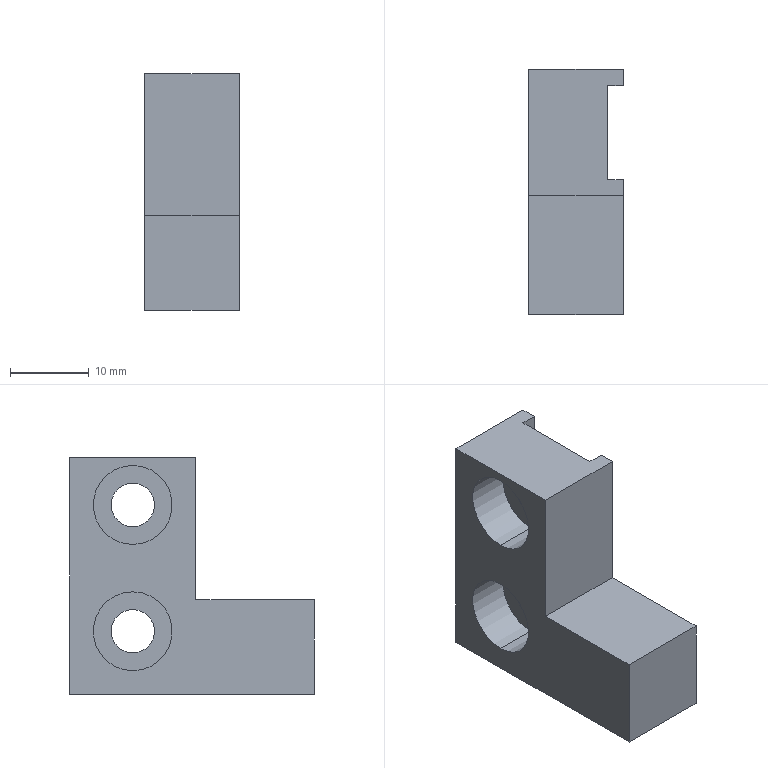Part | STEP file | PN_0009 | 1 solid | 22 faces | box 12 x 31 x 30 mm | volume 6133 mm3 | plane 14 | cylinder 8 | commonest cylinder face diameters 5.5 x4 10 x4